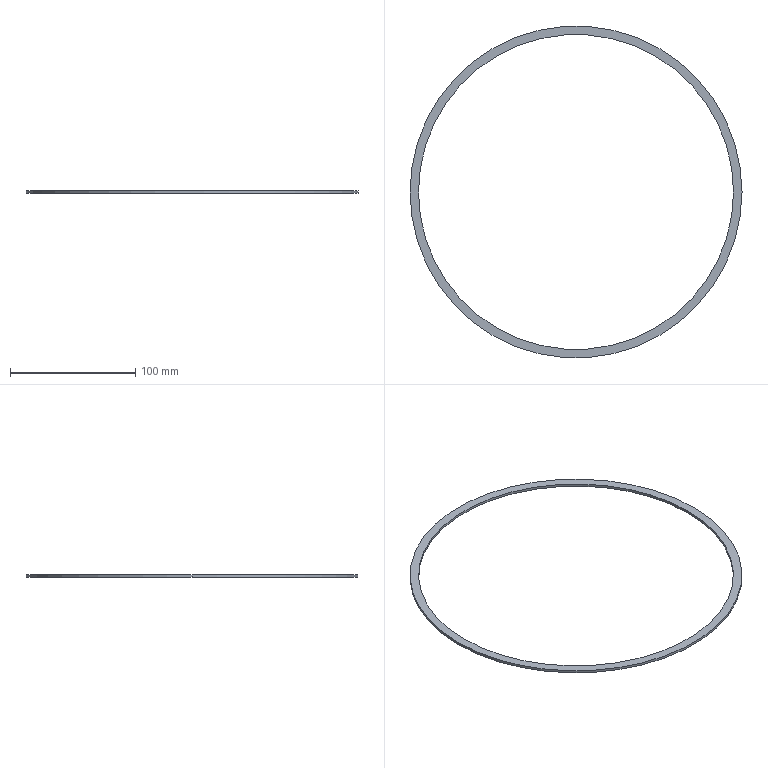Part | STEP file | EFXU21626_2 | 1 solid | 6 faces | box 264.6 x 264.6 x 2 mm | volume 11015 mm3 | cylinder 4 | plane 2 | commonest cylinder face diameters 251 x2 264.6 x2
STEP:
#1=CARTESIAN_POINT('',(0.,0.,0.));
#2=DIRECTION('',(0.,0.,1.));
#3=DIRECTION('',(1.,0.,0.));
#4=AXIS2_PLACEMENT_3D('',#1,#2,#3);
#5=CARTESIAN_POINT('',(-132.3,0.,2.7));
#6=VERTEX_POINT('',#5);
#7=CARTESIAN_POINT('',(132.3,0.,2.7));
#8=VERTEX_POINT('',#7);
#9=CARTESIAN_POINT('',(0.,0.,2.7));
#10=DIRECTION('',(0.,0.,-1.));
#11=DIRECTION('',(-1.,0.,0.));
#12=AXIS2_PLACEMENT_3D('',#9,#10,#11);
#13=CIRCLE('',#12,132.3);
#14=CARTESIAN_POINT('',(0.,0.,2.7));
#15=DIRECTION('',(0.,0.,-1.));
#16=DIRECTION('',(-1.,0.,0.));
#17=AXIS2_PLACEMENT_3D('',#14,#15,#16);
#18=CYLINDRICAL_SURFACE('',#17,132.3);
#19=CARTESIAN_POINT('',(0.,0.));
#20=DIRECTION('',(1.,0.));
#21=VECTOR('',#20,1.);
#22=LINE('',#19,#21);
#23=(GEOMETRIC_REPRESENTATION_CONTEXT(2)PARAMETRIC_REPRESENTATION_CONTEXT()REPRESENTATION_CONTEXT('',''));
#24=DEFINITIONAL_REPRESENTATION('',(#22),#23);
#25=PCURVE('',#18,#24);
#26=CARTESIAN_POINT('',(0.,0.,2.7));
#27=DIRECTION('',(0.,0.,-1.));
#28=DIRECTION('',(-1.,0.,0.));
#29=AXIS2_PLACEMENT_3D('',#26,#27,#28);
#30=PLANE('',#29);
#31=CARTESIAN_POINT('',(0.,0.));
#32=DIRECTION('',(1.,0.));
#33=AXIS2_PLACEMENT_2D('',#31,#32);
#34=CIRCLE('',#33,132.3);
#35=(GEOMETRIC_REPRESENTATION_CONTEXT(2)PARAMETRIC_REPRESENTATION_CONTEXT()REPRESENTATION_CONTEXT('',''));
#36=DEFINITIONAL_REPRESENTATION('',(#34),#35);
#37=PCURVE('',#30,#36);
#38=SURFACE_CURVE('',#13,(#25,#37),.PCURVE_S1.);
#39=EDGE_CURVE('',#6,#8,#38,.T.);
#40=ORIENTED_EDGE('',*,*,#39,.T.);
#41=CARTESIAN_POINT('',(132.3,0.,0.7));
#42=VERTEX_POINT('',#41);
#43=CARTESIAN_POINT('',(132.3,0.,2.7));
#44=DIRECTION('',(0.,0.,-1.));
#45=VECTOR('',#44,1.);
#46=LINE('',#43,#45);
#47=CARTESIAN_POINT('',(3.142,0.));
#48=DIRECTION('',(0.,1.));
#49=VECTOR('',#48,1.);
#50=LINE('',#47,#49);
#51=(GEOMETRIC_REPRESENTATION_CONTEXT(2)PARAMETRIC_REPRESENTATION_CONTEXT()REPRESENTATION_CONTEXT('',''));
#52=DEFINITIONAL_REPRESENTATION('',(#50),#51);
#53=PCURVE('',#18,#52);
#54=CARTESIAN_POINT('',(0.,0.,2.7));
#55=DIRECTION('',(0.,0.,-1.));
#56=DIRECTION('',(-1.,0.,0.));
#57=AXIS2_PLACEMENT_3D('',#54,#55,#56);
#58=CYLINDRICAL_SURFACE('',#57,132.3);
#59=CARTESIAN_POINT('',(3.142,0.));
#60=DIRECTION('',(0.,1.));
#61=VECTOR('',#60,1.);
#62=LINE('',#59,#61);
#63=(GEOMETRIC_REPRESENTATION_CONTEXT(2)PARAMETRIC_REPRESENTATION_CONTEXT()REPRESENTATION_CONTEXT('',''));
#64=DEFINITIONAL_REPRESENTATION('',(#62),#63);
#65=PCURVE('',#58,#64);
#66=SURFACE_CURVE('',#46,(#53,#65),.PCURVE_S1.);
#67=EDGE_CURVE('',#8,#42,#66,.T.);
#68=ORIENTED_EDGE('',*,*,#67,.T.);
#69=CARTESIAN_POINT('',(-132.3,0.,0.7));
#70=VERTEX_POINT('',#69);
#71=CARTESIAN_POINT('',(0.,0.,0.7));
#72=DIRECTION('',(0.,0.,1.));
#73=DIRECTION('',(-1.,0.,0.));
#74=AXIS2_PLACEMENT_3D('',#71,#72,#73);
#75=CIRCLE('',#74,132.3);
#76=CARTESIAN_POINT('',(6.283,2.));
#77=DIRECTION('',(-1.,0.));
#78=VECTOR('',#77,1.);
#79=LINE('',#76,#78);
#80=(GEOMETRIC_REPRESENTATION_CONTEXT(2)PARAMETRIC_REPRESENTATION_CONTEXT()REPRESENTATION_CONTEXT('',''));
#81=DEFINITIONAL_REPRESENTATION('',(#79),#80);
#82=PCURVE('',#18,#81);
#83=CARTESIAN_POINT('',(0.,0.,0.7));
#84=DIRECTION('',(0.,0.,-1.));
#85=DIRECTION('',(-1.,0.,0.));
#86=AXIS2_PLACEMENT_3D('',#83,#84,#85);
#87=PLANE('',#86);
#88=CARTESIAN_POINT('',(132.3,0.));
#89=CARTESIAN_POINT('',(132.3,-229.15));
#90=CARTESIAN_POINT('',(-66.15,-114.575));
#91=CARTESIAN_POINT('',(-264.6,0.));
#92=CARTESIAN_POINT('',(-66.15,114.575));
#93=CARTESIAN_POINT('',(132.3,229.15));
#94=CARTESIAN_POINT('',(132.3,0.));
#95=(BOUNDED_CURVE()B_SPLINE_CURVE(2,(#88,#89,#90,#91,#92,#93,#94),.UNSPECIFIED.,.T.,.F.)B_SPLINE_CURVE_WITH_KNOTS((1,2,2,2,2,1),(-2.094,0.,2.094,4.189,6.283,8.378),.UNSPECIFIED.)CURVE()GEOMETRIC_REPRESENTATION_ITEM()RATIONAL_B_SPLINE_CURVE((1.,0.5,1.,0.5,1.,0.5,1.))REPRESENTATION_ITEM(''));
#96=(GEOMETRIC_REPRESENTATION_CONTEXT(2)PARAMETRIC_REPRESENTATION_CONTEXT()REPRESENTATION_CONTEXT('',''));
#97=DEFINITIONAL_REPRESENTATION('',(#95),#96);
#98=PCURVE('',#87,#97);
#99=SURFACE_CURVE('',#75,(#82,#98),.PCURVE_S1.);
#100=EDGE_CURVE('',#42,#70,#99,.T.);
#101=ORIENTED_EDGE('',*,*,#100,.T.);
#102=CARTESIAN_POINT('',(-132.3,0.,2.7));
#103=DIRECTION('',(0.,0.,-1.));
#104=VECTOR('',#103,1.);
#105=LINE('',#102,#104);
#106=CARTESIAN_POINT('',(0.,0.));
#107=DIRECTION('',(0.,1.));
#108=VECTOR('',#107,1.);
#109=LINE('',#106,#108);
#110=(GEOMETRIC_REPRESENTATION_CONTEXT(2)PARAMETRIC_REPRESENTATION_CONTEXT()REPRESENTATION_CONTEXT('',''));
#111=DEFINITIONAL_REPRESENTATION('',(#109),#110);
#112=PCURVE('',#18,#111);
#113=CARTESIAN_POINT('',(6.283,0.));
#114=DIRECTION('',(0.,1.));
#115=VECTOR('',#114,1.);
#116=LINE('',#113,#115);
#117=(GEOMETRIC_REPRESENTATION_CONTEXT(2)PARAMETRIC_REPRESENTATION_CONTEXT()REPRESENTATION_CONTEXT('',''));
#118=DEFINITIONAL_REPRESENTATION('',(#116),#117);
#119=PCURVE('',#58,#118);
#120=SURFACE_CURVE('',#105,(#112,#119),.PCURVE_S1.);
#121=EDGE_CURVE('',#6,#70,#120,.T.);
#122=ORIENTED_EDGE('',*,*,#121,.F.);
#123=EDGE_LOOP('',(#40,#68,#101,#122));
#124=FACE_BOUND('',#123,.T.);
#125=ADVANCED_FACE('',(#124),#18,.T.);
#126=CARTESIAN_POINT('',(-125.5,0.,2.7));
#127=VERTEX_POINT('',#126);
#128=CARTESIAN_POINT('',(-125.5,0.,0.7));
#129=VERTEX_POINT('',#128);
#130=CARTESIAN_POINT('',(-125.5,0.,2.7));
#131=DIRECTION('',(0.,0.,-1.));
#132=VECTOR('',#131,1.);
#133=LINE('',#130,#132);
#134=CARTESIAN_POINT('',(0.,0.,2.7));
#135=DIRECTION('',(0.,0.,-1.));
#136=DIRECTION('',(-1.,0.,0.));
#137=AXIS2_PLACEMENT_3D('',#134,#135,#136);
#138=CYLINDRICAL_SURFACE('',#137,125.5);
#139=CARTESIAN_POINT('',(6.283,0.));
#140=DIRECTION('',(0.,1.));
#141=VECTOR('',#140,1.);
#142=LINE('',#139,#141);
#143=(GEOMETRIC_REPRESENTATION_CONTEXT(2)PARAMETRIC_REPRESENTATION_CONTEXT()REPRESENTATION_CONTEXT('',''));
#144=DEFINITIONAL_REPRESENTATION('',(#142),#143);
#145=PCURVE('',#138,#144);
#146=CARTESIAN_POINT('',(0.,0.,2.7));
#147=DIRECTION('',(0.,0.,-1.));
#148=DIRECTION('',(-1.,0.,0.));
#149=AXIS2_PLACEMENT_3D('',#146,#147,#148);
#150=CYLINDRICAL_SURFACE('',#149,125.5);
#151=CARTESIAN_POINT('',(0.,0.));
#152=DIRECTION('',(0.,1.));
#153=VECTOR('',#152,1.);
#154=LINE('',#151,#153);
#155=(GEOMETRIC_REPRESENTATION_CONTEXT(2)PARAMETRIC_REPRESENTATION_CONTEXT()REPRESENTATION_CONTEXT('',''));
#156=DEFINITIONAL_REPRESENTATION('',(#154),#155);
#157=PCURVE('',#150,#156);
#158=SURFACE_CURVE('',#133,(#145,#157),.PCURVE_S1.);
#159=EDGE_CURVE('',#127,#129,#158,.T.);
#160=ORIENTED_EDGE('',*,*,#159,.T.);
#161=CARTESIAN_POINT('',(125.5,0.,0.7));
#162=VERTEX_POINT('',#161);
#163=CARTESIAN_POINT('',(0.,0.,0.7));
#164=DIRECTION('',(0.,0.,1.));
#165=DIRECTION('',(-1.,0.,0.));
#166=AXIS2_PLACEMENT_3D('',#163,#164,#165);
#167=CIRCLE('',#166,125.5);
#168=CARTESIAN_POINT('',(6.283,2.));
#169=DIRECTION('',(-1.,0.));
#170=VECTOR('',#169,1.);
#171=LINE('',#168,#170);
#172=(GEOMETRIC_REPRESENTATION_CONTEXT(2)PARAMETRIC_REPRESENTATION_CONTEXT()REPRESENTATION_CONTEXT('',''));
#173=DEFINITIONAL_REPRESENTATION('',(#171),#172);
#174=PCURVE('',#138,#173);
#175=CARTESIAN_POINT('',(125.5,0.));
#176=CARTESIAN_POINT('',(125.5,-217.372));
#177=CARTESIAN_POINT('',(-62.75,-108.686));
#178=CARTESIAN_POINT('',(-251.,0.));
#179=CARTESIAN_POINT('',(-62.75,108.686));
#180=CARTESIAN_POINT('',(125.5,217.372));
#181=CARTESIAN_POINT('',(125.5,0.));
#182=(BOUNDED_CURVE()B_SPLINE_CURVE(2,(#175,#176,#177,#178,#179,#180,#181),.UNSPECIFIED.,.T.,.F.)B_SPLINE_CURVE_WITH_KNOTS((1,2,2,2,2,1),(-2.094,0.,2.094,4.189,6.283,8.378),.UNSPECIFIED.)CURVE()GEOMETRIC_REPRESENTATION_ITEM()RATIONAL_B_SPLINE_CURVE((1.,0.5,1.,0.5,1.,0.5,1.))REPRESENTATION_ITEM(''));
#183=(GEOMETRIC_REPRESENTATION_CONTEXT(2)PARAMETRIC_REPRESENTATION_CONTEXT()REPRESENTATION_CONTEXT('',''));
#184=DEFINITIONAL_REPRESENTATION('',(#182),#183);
#185=PCURVE('',#87,#184);
#186=SURFACE_CURVE('',#167,(#174,#185),.PCURVE_S1.);
#187=EDGE_CURVE('',#129,#162,#186,.T.);
#188=ORIENTED_EDGE('',*,*,#187,.T.);
#189=CARTESIAN_POINT('',(125.5,0.,2.7));
#190=VERTEX_POINT('',#189);
#191=CARTESIAN_POINT('',(125.5,0.,2.7));
#192=DIRECTION('',(0.,0.,-1.));
#193=VECTOR('',#192,1.);
#194=LINE('',#191,#193);
#195=CARTESIAN_POINT('',(3.142,0.));
#196=DIRECTION('',(0.,1.));
#197=VECTOR('',#196,1.);
#198=LINE('',#195,#197);
#199=(GEOMETRIC_REPRESENTATION_CONTEXT(2)PARAMETRIC_REPRESENTATION_CONTEXT()REPRESENTATION_CONTEXT('',''));
#200=DEFINITIONAL_REPRESENTATION('',(#198),#199);
#201=PCURVE('',#138,#200);
#202=CARTESIAN_POINT('',(3.142,0.));
#203=DIRECTION('',(0.,1.));
#204=VECTOR('',#203,1.);
#205=LINE('',#202,#204);
#206=(GEOMETRIC_REPRESENTATION_CONTEXT(2)PARAMETRIC_REPRESENTATION_CONTEXT()REPRESENTATION_CONTEXT('',''));
#207=DEFINITIONAL_REPRESENTATION('',(#205),#206);
#208=PCURVE('',#150,#207);
#209=SURFACE_CURVE('',#194,(#201,#208),.PCURVE_S1.);
#210=EDGE_CURVE('',#190,#162,#209,.T.);
#211=ORIENTED_EDGE('',*,*,#210,.F.);
#212=CARTESIAN_POINT('',(0.,0.,2.7));
#213=DIRECTION('',(0.,0.,1.));
#214=DIRECTION('',(-1.,0.,0.));
#215=AXIS2_PLACEMENT_3D('',#212,#213,#214);
#216=CIRCLE('',#215,125.5);
#217=CARTESIAN_POINT('',(6.283,0.));
#218=DIRECTION('',(-1.,0.));
#219=VECTOR('',#218,1.);
#220=LINE('',#217,#219);
#221=(GEOMETRIC_REPRESENTATION_CONTEXT(2)PARAMETRIC_REPRESENTATION_CONTEXT()REPRESENTATION_CONTEXT('',''));
#222=DEFINITIONAL_REPRESENTATION('',(#220),#221);
#223=PCURVE('',#138,#222);
#224=CARTESIAN_POINT('',(125.5,0.));
#225=CARTESIAN_POINT('',(125.5,-217.372));
#226=CARTESIAN_POINT('',(-62.75,-108.686));
#227=CARTESIAN_POINT('',(-251.,0.));
#228=CARTESIAN_POINT('',(-62.75,108.686));
#229=CARTESIAN_POINT('',(125.5,217.372));
#230=CARTESIAN_POINT('',(125.5,0.));
#231=(BOUNDED_CURVE()B_SPLINE_CURVE(2,(#224,#225,#226,#227,#228,#229,#230),.UNSPECIFIED.,.T.,.F.)B_SPLINE_CURVE_WITH_KNOTS((1,2,2,2,2,1),(-2.094,0.,2.094,4.189,6.283,8.378),.UNSPECIFIED.)CURVE()GEOMETRIC_REPRESENTATION_ITEM()RATIONAL_B_SPLINE_CURVE((1.,0.5,1.,0.5,1.,0.5,1.))REPRESENTATION_ITEM(''));
#232=(GEOMETRIC_REPRESENTATION_CONTEXT(2)PARAMETRIC_REPRESENTATION_CONTEXT()REPRESENTATION_CONTEXT('',''));
#233=DEFINITIONAL_REPRESENTATION('',(#231),#232);
#234=PCURVE('',#30,#233);
#235=SURFACE_CURVE('',#216,(#223,#234),.PCURVE_S1.);
#236=EDGE_CURVE('',#127,#190,#235,.T.);
#237=ORIENTED_EDGE('',*,*,#236,.F.);
#238=EDGE_LOOP('',(#160,#188,#211,#237));
#239=FACE_BOUND('',#238,.F.);
#240=ADVANCED_FACE('',(#239),#138,.F.);
#241=ORIENTED_EDGE('',*,*,#39,.F.);
#242=CARTESIAN_POINT('',(0.,0.,2.7));
#243=DIRECTION('',(0.,0.,-1.));
#244=DIRECTION('',(-1.,0.,0.));
#245=AXIS2_PLACEMENT_3D('',#242,#243,#244);
#246=CIRCLE('',#245,132.3);
#247=CARTESIAN_POINT('',(0.,0.));
#248=DIRECTION('',(1.,0.));
#249=AXIS2_PLACEMENT_2D('',#247,#248);
#250=CIRCLE('',#249,132.3);
#251=(GEOMETRIC_REPRESENTATION_CONTEXT(2)PARAMETRIC_REPRESENTATION_CONTEXT()REPRESENTATION_CONTEXT('',''));
#252=DEFINITIONAL_REPRESENTATION('',(#250),#251);
#253=PCURVE('',#30,#252);
#254=CARTESIAN_POINT('',(0.,0.));
#255=DIRECTION('',(1.,0.));
#256=VECTOR('',#255,1.);
#257=LINE('',#254,#256);
#258=(GEOMETRIC_REPRESENTATION_CONTEXT(2)PARAMETRIC_REPRESENTATION_CONTEXT()REPRESENTATION_CONTEXT('',''));
#259=DEFINITIONAL_REPRESENTATION('',(#257),#258);
#260=PCURVE('',#58,#259);
#261=SURFACE_CURVE('',#246,(#253,#260),.PCURVE_S1.);
#262=EDGE_CURVE('',#8,#6,#261,.T.);
#263=ORIENTED_EDGE('',*,*,#262,.F.);
#264=EDGE_LOOP('',(#241,#263));
#265=FACE_BOUND('',#264,.T.);
#266=ORIENTED_EDGE('',*,*,#236,.F.);
#267=CARTESIAN_POINT('',(0.,0.,2.7));
#268=DIRECTION('',(0.,0.,1.));
#269=DIRECTION('',(-1.,0.,0.));
#270=AXIS2_PLACEMENT_3D('',#267,#268,#269);
#271=CIRCLE('',#270,125.5);
#272=CARTESIAN_POINT('',(125.5,0.));
#273=CARTESIAN_POINT('',(125.5,-217.372));
#274=CARTESIAN_POINT('',(-62.75,-108.686));
#275=CARTESIAN_POINT('',(-251.,0.));
#276=CARTESIAN_POINT('',(-62.75,108.686));
#277=CARTESIAN_POINT('',(125.5,217.372));
#278=CARTESIAN_POINT('',(125.5,0.));
#279=(BOUNDED_CURVE()B_SPLINE_CURVE(2,(#272,#273,#274,#275,#276,#277,#278),.UNSPECIFIED.,.T.,.F.)B_SPLINE_CURVE_WITH_KNOTS((1,2,2,2,2,1),(-2.094,0.,2.094,4.189,6.283,8.378),.UNSPECIFIED.)CURVE()GEOMETRIC_REPRESENTATION_ITEM()RATIONAL_B_SPLINE_CURVE((1.,0.5,1.,0.5,1.,0.5,1.))REPRESENTATION_ITEM(''));
#280=(GEOMETRIC_REPRESENTATION_CONTEXT(2)PARAMETRIC_REPRESENTATION_CONTEXT()REPRESENTATION_CONTEXT('',''));
#281=DEFINITIONAL_REPRESENTATION('',(#279),#280);
#282=PCURVE('',#30,#281);
#283=CARTESIAN_POINT('',(6.283,0.));
#284=DIRECTION('',(-1.,0.));
#285=VECTOR('',#284,1.);
#286=LINE('',#283,#285);
#287=(GEOMETRIC_REPRESENTATION_CONTEXT(2)PARAMETRIC_REPRESENTATION_CONTEXT()REPRESENTATION_CONTEXT('',''));
#288=DEFINITIONAL_REPRESENTATION('',(#286),#287);
#289=PCURVE('',#150,#288);
#290=SURFACE_CURVE('',#271,(#282,#289),.PCURVE_S1.);
#291=EDGE_CURVE('',#190,#127,#290,.T.);
#292=ORIENTED_EDGE('',*,*,#291,.F.);
#293=EDGE_LOOP('',(#266,#292));
#294=FACE_BOUND('',#293,.T.);
#295=ADVANCED_FACE('',(#265,#294),#30,.F.);
#296=ORIENTED_EDGE('',*,*,#67,.F.);
#297=ORIENTED_EDGE('',*,*,#262,.T.);
#298=ORIENTED_EDGE('',*,*,#121,.T.);
#299=CARTESIAN_POINT('',(0.,0.,0.7));
#300=DIRECTION('',(0.,0.,1.));
#301=DIRECTION('',(-1.,0.,0.));
#302=AXIS2_PLACEMENT_3D('',#299,#300,#301);
#303=CIRCLE('',#302,132.3);
#304=CARTESIAN_POINT('',(6.283,2.));
#305=DIRECTION('',(-1.,0.));
#306=VECTOR('',#305,1.);
#307=LINE('',#304,#306);
#308=(GEOMETRIC_REPRESENTATION_CONTEXT(2)PARAMETRIC_REPRESENTATION_CONTEXT()REPRESENTATION_CONTEXT('',''));
#309=DEFINITIONAL_REPRESENTATION('',(#307),#308);
#310=PCURVE('',#58,#309);
#311=CARTESIAN_POINT('',(132.3,0.));
#312=CARTESIAN_POINT('',(132.3,-229.15));
#313=CARTESIAN_POINT('',(-66.15,-114.575));
#314=CARTESIAN_POINT('',(-264.6,0.));
#315=CARTESIAN_POINT('',(-66.15,114.575));
#316=CARTESIAN_POINT('',(132.3,229.15));
#317=CARTESIAN_POINT('',(132.3,0.));
#318=(BOUNDED_CURVE()B_SPLINE_CURVE(2,(#311,#312,#313,#314,#315,#316,#317),.UNSPECIFIED.,.T.,.F.)B_SPLINE_CURVE_WITH_KNOTS((1,2,2,2,2,1),(-2.094,0.,2.094,4.189,6.283,8.378),.UNSPECIFIED.)CURVE()GEOMETRIC_REPRESENTATION_ITEM()RATIONAL_B_SPLINE_CURVE((1.,0.5,1.,0.5,1.,0.5,1.))REPRESENTATION_ITEM(''));
#319=(GEOMETRIC_REPRESENTATION_CONTEXT(2)PARAMETRIC_REPRESENTATION_CONTEXT()REPRESENTATION_CONTEXT('',''));
#320=DEFINITIONAL_REPRESENTATION('',(#318),#319);
#321=PCURVE('',#87,#320);
#322=SURFACE_CURVE('',#303,(#310,#321),.PCURVE_S1.);
#323=EDGE_CURVE('',#70,#42,#322,.T.);
#324=ORIENTED_EDGE('',*,*,#323,.T.);
#325=EDGE_LOOP('',(#296,#297,#298,#324));
#326=FACE_BOUND('',#325,.T.);
#327=ADVANCED_FACE('',(#326),#58,.T.);
#328=CARTESIAN_POINT('',(0.,0.,0.7));
#329=DIRECTION('',(0.,0.,1.));
#330=DIRECTION('',(-1.,0.,0.));
#331=AXIS2_PLACEMENT_3D('',#328,#329,#330);
#332=CIRCLE('',#331,125.5);
#333=CARTESIAN_POINT('',(6.283,2.));
#334=DIRECTION('',(-1.,0.));
#335=VECTOR('',#334,1.);
#336=LINE('',#333,#335);
#337=(GEOMETRIC_REPRESENTATION_CONTEXT(2)PARAMETRIC_REPRESENTATION_CONTEXT()REPRESENTATION_CONTEXT('',''));
#338=DEFINITIONAL_REPRESENTATION('',(#336),#337);
#339=PCURVE('',#150,#338);
#340=CARTESIAN_POINT('',(125.5,0.));
#341=CARTESIAN_POINT('',(125.5,-217.372));
#342=CARTESIAN_POINT('',(-62.75,-108.686));
#343=CARTESIAN_POINT('',(-251.,0.));
#344=CARTESIAN_POINT('',(-62.75,108.686));
#345=CARTESIAN_POINT('',(125.5,217.372));
#346=CARTESIAN_POINT('',(125.5,0.));
#347=(BOUNDED_CURVE()B_SPLINE_CURVE(2,(#340,#341,#342,#343,#344,#345,#346),.UNSPECIFIED.,.T.,.F.)B_SPLINE_CURVE_WITH_KNOTS((1,2,2,2,2,1),(-2.094,0.,2.094,4.189,6.283,8.378),.UNSPECIFIED.)CURVE()GEOMETRIC_REPRESENTATION_ITEM()RATIONAL_B_SPLINE_CURVE((1.,0.5,1.,0.5,1.,0.5,1.))REPRESENTATION_ITEM(''));
#348=(GEOMETRIC_REPRESENTATION_CONTEXT(2)PARAMETRIC_REPRESENTATION_CONTEXT()REPRESENTATION_CONTEXT('',''));
#349=DEFINITIONAL_REPRESENTATION('',(#347),#348);
#350=PCURVE('',#87,#349);
#351=SURFACE_CURVE('',#332,(#339,#350),.PCURVE_S1.);
#352=EDGE_CURVE('',#162,#129,#351,.T.);
#353=ORIENTED_EDGE('',*,*,#352,.T.);
#354=ORIENTED_EDGE('',*,*,#159,.F.);
#355=ORIENTED_EDGE('',*,*,#291,.F.);
#356=ORIENTED_EDGE('',*,*,#210,.T.);
#357=EDGE_LOOP('',(#353,#354,#355,#356));
#358=FACE_BOUND('',#357,.F.);
#359=ADVANCED_FACE('',(#358),#150,.F.);
#360=ORIENTED_EDGE('',*,*,#323,.F.);
#361=ORIENTED_EDGE('',*,*,#100,.F.);
#362=EDGE_LOOP('',(#360,#361));
#363=FACE_BOUND('',#362,.T.);
#364=ORIENTED_EDGE('',*,*,#187,.T.);
#365=ORIENTED_EDGE('',*,*,#352,.T.);
#366=EDGE_LOOP('',(#364,#365));
#367=FACE_BOUND('',#366,.T.);
#368=ADVANCED_FACE('',(#363,#367),#87,.T.);
#369=CLOSED_SHELL('',(#125,#240,#295,#327,#359,#368));
#370=MANIFOLD_SOLID_BREP('',#369);
#371=(LENGTH_UNIT()NAMED_UNIT(*)SI_UNIT(.MILLI.,.METRE.));
#372=UNCERTAINTY_MEASURE_WITH_UNIT(LENGTH_MEASURE(0.0000001),#371,'','');
#373=(NAMED_UNIT(*)PLANE_ANGLE_UNIT()SI_UNIT($,.RADIAN.));
#374=(NAMED_UNIT(*)SI_UNIT($,.STERADIAN.)SOLID_ANGLE_UNIT());
#375=(GEOMETRIC_REPRESENTATION_CONTEXT(3)GLOBAL_UNCERTAINTY_ASSIGNED_CONTEXT((#372))GLOBAL_UNIT_ASSIGNED_CONTEXT((#371,#373,#374))REPRESENTATION_CONTEXT('',''));
#376=ADVANCED_BREP_SHAPE_REPRESENTATION('',(#4,#370),#375);